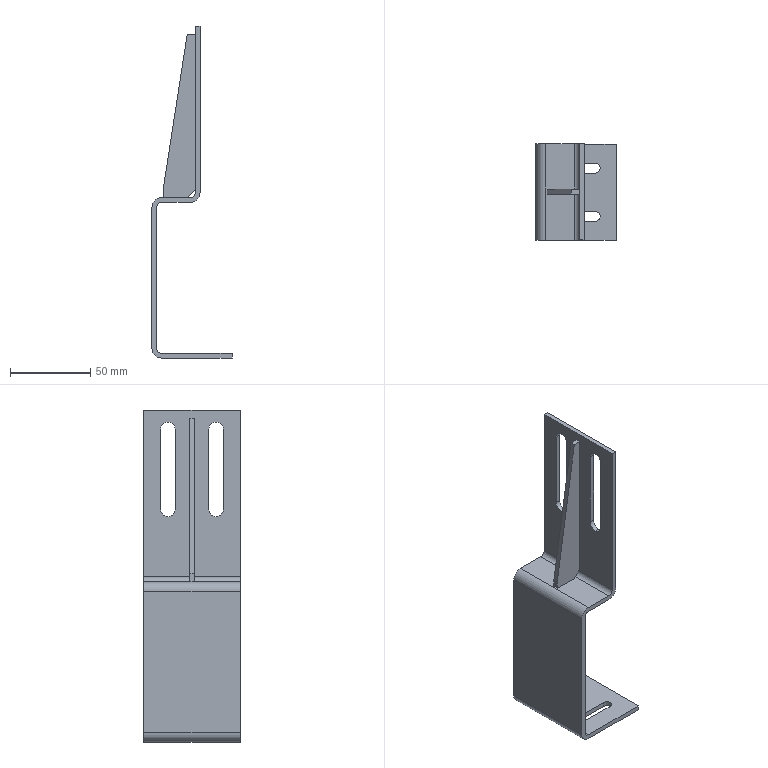Part | SolidWorks | features BaseBody 1 | 1 solid | 44 faces | box 50 x 60 x 207 mm | volume 49322 mm3 | plane 26 | cylinder 18 | commonest cylinder face diameters 6 x9 9 x6 12 x3
STEP:
#1=CARTESIAN_POINT('',(10.,15.,-97.));
#2=VERTEX_POINT('',#1);
#3=CARTESIAN_POINT('',(13.,18.,-97.));
#4=VERTEX_POINT('',#3);
#5=CARTESIAN_POINT('',(13.,15.,-97.));
#6=DIRECTION('',(0.,0.,-1.));
#7=DIRECTION('',(-1.,0.,0.));
#8=AXIS2_PLACEMENT_3D('',#5,#6,#7);
#9=CIRCLE('',#8,3.);
#10=EDGE_CURVE('',#2,#4,#9,.T.);
#11=ORIENTED_EDGE('',*,*,#10,.F.);
#12=CARTESIAN_POINT('',(10.,15.,-100.));
#13=VERTEX_POINT('',#12);
#14=CARTESIAN_POINT('',(10.,15.,-100.));
#15=DIRECTION('',(0.,0.,-1.));
#16=VECTOR('',#15,1000.);
#17=LINE('',#14,#16);
#18=EDGE_CURVE('',#2,#13,#17,.T.);
#19=ORIENTED_EDGE('',*,*,#18,.T.);
#20=CARTESIAN_POINT('',(13.,18.,-100.));
#21=VERTEX_POINT('',#20);
#22=CARTESIAN_POINT('',(13.,15.,-100.));
#23=DIRECTION('',(0.,0.,1.));
#24=DIRECTION('',(-1.,0.,0.));
#25=AXIS2_PLACEMENT_3D('',#22,#23,#24);
#26=CIRCLE('',#25,3.);
#27=EDGE_CURVE('',#21,#13,#26,.T.);
#28=ORIENTED_EDGE('',*,*,#27,.F.);
#29=CARTESIAN_POINT('',(13.,18.,-100.));
#30=DIRECTION('',(0.,0.,1.));
#31=VECTOR('',#30,1000.);
#32=LINE('',#29,#31);
#33=EDGE_CURVE('',#21,#4,#32,.T.);
#34=ORIENTED_EDGE('',*,*,#33,.T.);
#35=EDGE_LOOP('',(#11,#19,#28,#34));
#36=FACE_OUTER_BOUND('',#35,.T.);
#37=CARTESIAN_POINT('',(13.,15.,-100.));
#38=DIRECTION('',(0.,0.,-1.));
#39=DIRECTION('',(-1.,0.,0.));
#40=AXIS2_PLACEMENT_3D('',#37,#38,#39);
#41=CYLINDRICAL_SURFACE('',#40,3.);
#42=ADVANCED_FACE('',(#36),#41,.F.);
#43=CARTESIAN_POINT('',(10.,-15.,-97.));
#44=VERTEX_POINT('',#43);
#45=CARTESIAN_POINT('',(13.,-12.,-97.));
#46=VERTEX_POINT('',#45);
#47=CARTESIAN_POINT('',(13.,-15.,-97.));
#48=DIRECTION('',(0.,0.,-1.));
#49=DIRECTION('',(-1.,0.,0.));
#50=AXIS2_PLACEMENT_3D('',#47,#48,#49);
#51=CIRCLE('',#50,3.);
#52=EDGE_CURVE('',#44,#46,#51,.T.);
#53=ORIENTED_EDGE('',*,*,#52,.F.);
#54=CARTESIAN_POINT('',(10.,-15.,-100.));
#55=VERTEX_POINT('',#54);
#56=CARTESIAN_POINT('',(10.,-15.,-100.));
#57=DIRECTION('',(0.,0.,-1.));
#58=VECTOR('',#57,1000.);
#59=LINE('',#56,#58);
#60=EDGE_CURVE('',#44,#55,#59,.T.);
#61=ORIENTED_EDGE('',*,*,#60,.T.);
#62=CARTESIAN_POINT('',(13.,-12.,-100.));
#63=VERTEX_POINT('',#62);
#64=CARTESIAN_POINT('',(13.,-15.,-100.));
#65=DIRECTION('',(0.,0.,1.));
#66=DIRECTION('',(-1.,0.,0.));
#67=AXIS2_PLACEMENT_3D('',#64,#65,#66);
#68=CIRCLE('',#67,3.);
#69=EDGE_CURVE('',#63,#55,#68,.T.);
#70=ORIENTED_EDGE('',*,*,#69,.F.);
#71=CARTESIAN_POINT('',(13.,-12.,-100.));
#72=DIRECTION('',(0.,0.,-1.));
#73=VECTOR('',#72,1000.);
#74=LINE('',#71,#73);
#75=EDGE_CURVE('',#46,#63,#74,.T.);
#76=ORIENTED_EDGE('',*,*,#75,.F.);
#77=EDGE_LOOP('',(#53,#61,#70,#76));
#78=FACE_OUTER_BOUND('',#77,.T.);
#79=CARTESIAN_POINT('',(13.,-15.,-100.));
#80=DIRECTION('',(0.,0.,-1.));
#81=DIRECTION('',(-1.,0.,0.));
#82=AXIS2_PLACEMENT_3D('',#79,#80,#81);
#83=CYLINDRICAL_SURFACE('',#82,3.);
#84=ADVANCED_FACE('',(#78),#83,.F.);
#85=CARTESIAN_POINT('',(27.,15.,40.5));
#86=VERTEX_POINT('',#85);
#87=CARTESIAN_POINT('',(27.,19.5,45.));
#88=VERTEX_POINT('',#87);
#89=CARTESIAN_POINT('',(27.,15.,45.));
#90=DIRECTION('',(1.,0.,0.));
#91=DIRECTION('',(0.,0.,-1.));
#92=AXIS2_PLACEMENT_3D('',#89,#90,#91);
#93=CIRCLE('',#92,4.5);
#94=EDGE_CURVE('',#86,#88,#93,.T.);
#95=ORIENTED_EDGE('',*,*,#94,.F.);
#96=CARTESIAN_POINT('',(30.,15.,40.5));
#97=VERTEX_POINT('',#96);
#98=CARTESIAN_POINT('',(30.,15.,40.5));
#99=DIRECTION('',(1.,0.,0.));
#100=VECTOR('',#99,1000.);
#101=LINE('',#98,#100);
#102=EDGE_CURVE('',#86,#97,#101,.T.);
#103=ORIENTED_EDGE('',*,*,#102,.T.);
#104=CARTESIAN_POINT('',(30.,19.5,45.));
#105=VERTEX_POINT('',#104);
#106=CARTESIAN_POINT('',(30.,15.,45.));
#107=DIRECTION('',(-1.,0.,0.));
#108=DIRECTION('',(0.,0.,-1.));
#109=AXIS2_PLACEMENT_3D('',#106,#107,#108);
#110=CIRCLE('',#109,4.5);
#111=EDGE_CURVE('',#105,#97,#110,.T.);
#112=ORIENTED_EDGE('',*,*,#111,.F.);
#113=CARTESIAN_POINT('',(30.,19.5,45.));
#114=DIRECTION('',(-1.,0.,0.));
#115=VECTOR('',#114,1000.);
#116=LINE('',#113,#115);
#117=EDGE_CURVE('',#105,#88,#116,.T.);
#118=ORIENTED_EDGE('',*,*,#117,.T.);
#119=EDGE_LOOP('',(#95,#103,#112,#118));
#120=FACE_OUTER_BOUND('',#119,.T.);
#121=CARTESIAN_POINT('',(30.,15.,45.));
#122=DIRECTION('',(1.,0.,0.));
#123=DIRECTION('',(0.,0.,-1.));
#124=AXIS2_PLACEMENT_3D('',#121,#122,#123);
#125=CYLINDRICAL_SURFACE('',#124,4.5);
#126=ADVANCED_FACE('',(#120),#125,.F.);
#127=CARTESIAN_POINT('',(27.,-15.,40.5));
#128=VERTEX_POINT('',#127);
#129=CARTESIAN_POINT('',(27.,-10.5,45.));
#130=VERTEX_POINT('',#129);
#131=CARTESIAN_POINT('',(27.,-15.,45.));
#132=DIRECTION('',(1.,0.,0.));
#133=DIRECTION('',(0.,0.,-1.));
#134=AXIS2_PLACEMENT_3D('',#131,#132,#133);
#135=CIRCLE('',#134,4.5);
#136=EDGE_CURVE('',#128,#130,#135,.T.);
#137=ORIENTED_EDGE('',*,*,#136,.F.);
#138=CARTESIAN_POINT('',(30.,-15.,40.5));
#139=VERTEX_POINT('',#138);
#140=CARTESIAN_POINT('',(30.,-15.,40.5));
#141=DIRECTION('',(1.,0.,0.));
#142=VECTOR('',#141,1000.);
#143=LINE('',#140,#142);
#144=EDGE_CURVE('',#128,#139,#143,.T.);
#145=ORIENTED_EDGE('',*,*,#144,.T.);
#146=CARTESIAN_POINT('',(30.,-10.5,45.));
#147=VERTEX_POINT('',#146);
#148=CARTESIAN_POINT('',(30.,-15.,45.));
#149=DIRECTION('',(-1.,0.,0.));
#150=DIRECTION('',(0.,0.,-1.));
#151=AXIS2_PLACEMENT_3D('',#148,#149,#150);
#152=CIRCLE('',#151,4.5);
#153=EDGE_CURVE('',#147,#139,#152,.T.);
#154=ORIENTED_EDGE('',*,*,#153,.F.);
#155=CARTESIAN_POINT('',(30.,-10.5,45.));
#156=DIRECTION('',(1.,0.,0.));
#157=VECTOR('',#156,1000.);
#158=LINE('',#155,#157);
#159=EDGE_CURVE('',#130,#147,#158,.T.);
#160=ORIENTED_EDGE('',*,*,#159,.F.);
#161=EDGE_LOOP('',(#137,#145,#154,#160));
#162=FACE_OUTER_BOUND('',#161,.T.);
#163=CARTESIAN_POINT('',(30.,-15.,45.));
#164=DIRECTION('',(1.,0.,0.));
#165=DIRECTION('',(0.,0.,-1.));
#166=AXIS2_PLACEMENT_3D('',#163,#164,#165);
#167=CYLINDRICAL_SURFACE('',#166,4.5);
#168=ADVANCED_FACE('',(#162),#167,.F.);
#169=CARTESIAN_POINT('',(0.,30.,-94.));
#170=VERTEX_POINT('',#169);
#171=CARTESIAN_POINT('',(0.,-30.,-94.));
#172=VERTEX_POINT('',#171);
#173=CARTESIAN_POINT('',(0.,-30.,-94.));
#174=DIRECTION('',(0.,-1.,0.));
#175=VECTOR('',#174,1000.);
#176=LINE('',#173,#175);
#177=EDGE_CURVE('',#170,#172,#176,.T.);
#178=ORIENTED_EDGE('',*,*,#177,.T.);
#179=CARTESIAN_POINT('',(0.,-30.,-6.));
#180=VERTEX_POINT('',#179);
#181=CARTESIAN_POINT('',(0.,-30.,-94.));
#182=DIRECTION('',(0.,0.,1.));
#183=VECTOR('',#182,1000.);
#184=LINE('',#181,#183);
#185=EDGE_CURVE('',#172,#180,#184,.T.);
#186=ORIENTED_EDGE('',*,*,#185,.T.);
#187=CARTESIAN_POINT('',(0.,30.,-6.));
#188=VERTEX_POINT('',#187);
#189=CARTESIAN_POINT('',(0.,-30.,-6.));
#190=DIRECTION('',(0.,1.,0.));
#191=VECTOR('',#190,1000.);
#192=LINE('',#189,#191);
#193=EDGE_CURVE('',#180,#188,#192,.T.);
#194=ORIENTED_EDGE('',*,*,#193,.T.);
#195=CARTESIAN_POINT('',(0.,30.,-94.));
#196=DIRECTION('',(0.,0.,-1.));
#197=VECTOR('',#196,1000.);
#198=LINE('',#195,#197);
#199=EDGE_CURVE('',#188,#170,#198,.T.);
#200=ORIENTED_EDGE('',*,*,#199,.T.);
#201=EDGE_LOOP('',(#178,#186,#194,#200));
#202=FACE_OUTER_BOUND('',#201,.T.);
#203=CARTESIAN_POINT('',(0.,-30.,-94.));
#204=DIRECTION('',(-1.,0.,0.));
#205=DIRECTION('',(0.,0.,1.));
#206=AXIS2_PLACEMENT_3D('',#203,#204,#205);
#207=PLANE('',#206);
#208=ADVANCED_FACE('',(#202),#207,.T.);
#209=CARTESIAN_POINT('',(6.,-30.,-100.));
#210=VERTEX_POINT('',#209);
#211=CARTESIAN_POINT('',(6.,-30.,-94.));
#212=DIRECTION('',(0.,1.,0.));
#213=DIRECTION('',(0.,0.,1.));
#214=AXIS2_PLACEMENT_3D('',#211,#212,#213);
#215=CIRCLE('',#214,6.);
#216=EDGE_CURVE('',#210,#172,#215,.T.);
#217=ORIENTED_EDGE('',*,*,#216,.F.);
#218=CARTESIAN_POINT('',(50.,-30.,-100.));
#219=VERTEX_POINT('',#218);
#220=CARTESIAN_POINT('',(0.,-30.,-100.));
#221=DIRECTION('',(-1.,0.,0.));
#222=VECTOR('',#221,1000.);
#223=LINE('',#220,#222);
#224=EDGE_CURVE('',#219,#210,#223,.T.);
#225=ORIENTED_EDGE('',*,*,#224,.F.);
#226=CARTESIAN_POINT('',(50.,-30.,-97.));
#227=VERTEX_POINT('',#226);
#228=CARTESIAN_POINT('',(50.,-30.,0.));
#229=DIRECTION('',(0.,0.,-1.));
#230=VECTOR('',#229,1000.);
#231=LINE('',#228,#230);
#232=EDGE_CURVE('',#227,#219,#231,.T.);
#233=ORIENTED_EDGE('',*,*,#232,.F.);
#234=CARTESIAN_POINT('',(6.,-30.,-97.));
#235=VERTEX_POINT('',#234);
#236=CARTESIAN_POINT('',(0.,-30.,-97.));
#237=DIRECTION('',(1.,0.,0.));
#238=VECTOR('',#237,1000.);
#239=LINE('',#236,#238);
#240=EDGE_CURVE('',#235,#227,#239,.T.);
#241=ORIENTED_EDGE('',*,*,#240,.F.);
#242=CARTESIAN_POINT('',(3.,-30.,-94.));
#243=VERTEX_POINT('',#242);
#244=CARTESIAN_POINT('',(6.,-30.,-94.));
#245=DIRECTION('',(0.,-1.,0.));
#246=DIRECTION('',(0.,0.,1.));
#247=AXIS2_PLACEMENT_3D('',#244,#245,#246);
#248=CIRCLE('',#247,3.);
#249=EDGE_CURVE('',#243,#235,#248,.T.);
#250=ORIENTED_EDGE('',*,*,#249,.F.);
#251=CARTESIAN_POINT('',(3.,-30.,-6.));
#252=VERTEX_POINT('',#251);
#253=CARTESIAN_POINT('',(3.,-30.,0.));
#254=DIRECTION('',(0.,0.,-1.));
#255=VECTOR('',#254,1000.);
#256=LINE('',#253,#255);
#257=EDGE_CURVE('',#252,#243,#256,.T.);
#258=ORIENTED_EDGE('',*,*,#257,.F.);
#259=CARTESIAN_POINT('',(6.,-30.,-3.));
#260=VERTEX_POINT('',#259);
#261=CARTESIAN_POINT('',(6.,-30.,-6.));
#262=DIRECTION('',(0.,-1.,0.));
#263=DIRECTION('',(0.,0.,1.));
#264=AXIS2_PLACEMENT_3D('',#261,#262,#263);
#265=CIRCLE('',#264,3.);
#266=EDGE_CURVE('',#260,#252,#265,.T.);
#267=ORIENTED_EDGE('',*,*,#266,.F.);
#268=CARTESIAN_POINT('',(24.,-30.,-3.));
#269=VERTEX_POINT('',#268);
#270=CARTESIAN_POINT('',(0.,-30.,-3.));
#271=DIRECTION('',(-1.,0.,0.));
#272=VECTOR('',#271,1000.);
#273=LINE('',#270,#272);
#274=EDGE_CURVE('',#269,#260,#273,.T.);
#275=ORIENTED_EDGE('',*,*,#274,.F.);
#276=CARTESIAN_POINT('',(30.,-30.,3.));
#277=VERTEX_POINT('',#276);
#278=CARTESIAN_POINT('',(24.,-30.,3.));
#279=DIRECTION('',(0.,1.,0.));
#280=DIRECTION('',(0.,0.,1.));
#281=AXIS2_PLACEMENT_3D('',#278,#279,#280);
#282=CIRCLE('',#281,6.);
#283=EDGE_CURVE('',#277,#269,#282,.T.);
#284=ORIENTED_EDGE('',*,*,#283,.F.);
#285=CARTESIAN_POINT('',(30.,-30.,107.));
#286=VERTEX_POINT('',#285);
#287=CARTESIAN_POINT('',(30.,-30.,0.));
#288=DIRECTION('',(0.,0.,-1.));
#289=VECTOR('',#288,1000.);
#290=LINE('',#287,#289);
#291=EDGE_CURVE('',#286,#277,#290,.T.);
#292=ORIENTED_EDGE('',*,*,#291,.F.);
#293=CARTESIAN_POINT('',(27.,-30.,107.));
#294=VERTEX_POINT('',#293);
#295=CARTESIAN_POINT('',(0.,-30.,107.));
#296=DIRECTION('',(1.,0.,0.));
#297=VECTOR('',#296,1000.);
#298=LINE('',#295,#297);
#299=EDGE_CURVE('',#294,#286,#298,.T.);
#300=ORIENTED_EDGE('',*,*,#299,.F.);
#301=CARTESIAN_POINT('',(27.,-30.,3.));
#302=VERTEX_POINT('',#301);
#303=CARTESIAN_POINT('',(27.,-30.,0.));
#304=DIRECTION('',(0.,0.,1.));
#305=VECTOR('',#304,1000.);
#306=LINE('',#303,#305);
#307=EDGE_CURVE('',#302,#294,#306,.T.);
#308=ORIENTED_EDGE('',*,*,#307,.F.);
#309=CARTESIAN_POINT('',(24.,-30.,0.));
#310=VERTEX_POINT('',#309);
#311=CARTESIAN_POINT('',(24.,-30.,3.));
#312=DIRECTION('',(0.,-1.,0.));
#313=DIRECTION('',(0.,0.,1.));
#314=AXIS2_PLACEMENT_3D('',#311,#312,#313);
#315=CIRCLE('',#314,3.);
#316=EDGE_CURVE('',#310,#302,#315,.T.);
#317=ORIENTED_EDGE('',*,*,#316,.F.);
#318=CARTESIAN_POINT('',(6.,-30.,0.));
#319=VERTEX_POINT('',#318);
#320=CARTESIAN_POINT('',(0.,-30.,0.));
#321=DIRECTION('',(1.,0.,0.));
#322=VECTOR('',#321,1000.);
#323=LINE('',#320,#322);
#324=EDGE_CURVE('',#319,#310,#323,.T.);
#325=ORIENTED_EDGE('',*,*,#324,.F.);
#326=CARTESIAN_POINT('',(6.,-30.,-6.));
#327=DIRECTION('',(0.,1.,0.));
#328=DIRECTION('',(0.,0.,1.));
#329=AXIS2_PLACEMENT_3D('',#326,#327,#328);
#330=CIRCLE('',#329,6.);
#331=EDGE_CURVE('',#180,#319,#330,.T.);
#332=ORIENTED_EDGE('',*,*,#331,.F.);
#333=ORIENTED_EDGE('',*,*,#185,.F.);
#334=EDGE_LOOP('',(#217,#225,#233,#241,#250,#258,#267,#275,#284,#292,#300,#308,#317,#325,#332,#333));
#335=FACE_OUTER_BOUND('',#334,.T.);
#336=CARTESIAN_POINT('',(0.,-30.,0.));
#337=DIRECTION('',(0.,1.,0.));
#338=DIRECTION('',(0.,0.,1.));
#339=AXIS2_PLACEMENT_3D('',#336,#337,#338);
#340=PLANE('',#339);
#341=ADVANCED_FACE('',(#335),#340,.F.);
#342=CARTESIAN_POINT('',(6.,30.,-100.));
#343=VERTEX_POINT('',#342);
#344=CARTESIAN_POINT('',(6.,-30.,-100.));
#345=DIRECTION('',(0.,-1.,0.));
#346=VECTOR('',#345,1000.);
#347=LINE('',#344,#346);
#348=EDGE_CURVE('',#343,#210,#347,.T.);
#349=ORIENTED_EDGE('',*,*,#348,.T.);
#350=ORIENTED_EDGE('',*,*,#216,.T.);
#351=ORIENTED_EDGE('',*,*,#177,.F.);
#352=CARTESIAN_POINT('',(6.,30.,-94.));
#353=DIRECTION('',(0.,-1.,0.));
#354=DIRECTION('',(0.,0.,1.));
#355=AXIS2_PLACEMENT_3D('',#352,#353,#354);
#356=CIRCLE('',#355,6.);
#357=EDGE_CURVE('',#170,#343,#356,.T.);
#358=ORIENTED_EDGE('',*,*,#357,.T.);
#359=EDGE_LOOP('',(#349,#350,#351,#358));
#360=FACE_OUTER_BOUND('',#359,.T.);
#361=CARTESIAN_POINT('',(6.,-30.,-94.));
#362=DIRECTION('',(0.,1.,0.));
#363=DIRECTION('',(0.,0.,1.));
#364=AXIS2_PLACEMENT_3D('',#361,#362,#363);
#365=CYLINDRICAL_SURFACE('',#364,6.);
#366=ADVANCED_FACE('',(#360),#365,.T.);
#367=ORIENTED_EDGE('',*,*,#199,.F.);
#368=CARTESIAN_POINT('',(6.,30.,0.));
#369=VERTEX_POINT('',#368);
#370=CARTESIAN_POINT('',(6.,30.,-6.));
#371=DIRECTION('',(0.,1.,0.));
#372=DIRECTION('',(0.,0.,1.));
#373=AXIS2_PLACEMENT_3D('',#370,#371,#372);
#374=CIRCLE('',#373,6.);
#375=EDGE_CURVE('',#188,#369,#374,.T.);
#376=ORIENTED_EDGE('',*,*,#375,.T.);
#377=CARTESIAN_POINT('',(24.,30.,0.));
#378=VERTEX_POINT('',#377);
#379=CARTESIAN_POINT('',(0.,30.,0.));
#380=DIRECTION('',(1.,0.,0.));
#381=VECTOR('',#380,1000.);
#382=LINE('',#379,#381);
#383=EDGE_CURVE('',#369,#378,#382,.T.);
#384=ORIENTED_EDGE('',*,*,#383,.T.);
#385=CARTESIAN_POINT('',(27.,30.,3.));
#386=VERTEX_POINT('',#385);
#387=CARTESIAN_POINT('',(24.,30.,3.));
#388=DIRECTION('',(0.,-1.,0.));
#389=DIRECTION('',(0.,0.,1.));
#390=AXIS2_PLACEMENT_3D('',#387,#388,#389);
#391=CIRCLE('',#390,3.);
#392=EDGE_CURVE('',#378,#386,#391,.T.);
#393=ORIENTED_EDGE('',*,*,#392,.T.);
#394=CARTESIAN_POINT('',(27.,30.,107.));
#395=VERTEX_POINT('',#394);
#396=CARTESIAN_POINT('',(27.,30.,0.));
#397=DIRECTION('',(0.,0.,1.));
#398=VECTOR('',#397,1000.);
#399=LINE('',#396,#398);
#400=EDGE_CURVE('',#386,#395,#399,.T.);
#401=ORIENTED_EDGE('',*,*,#400,.T.);
#402=CARTESIAN_POINT('',(30.,30.,107.));
#403=VERTEX_POINT('',#402);
#404=CARTESIAN_POINT('',(0.,30.,107.));
#405=DIRECTION('',(1.,0.,0.));
#406=VECTOR('',#405,1000.);
#407=LINE('',#404,#406);
#408=EDGE_CURVE('',#395,#403,#407,.T.);
#409=ORIENTED_EDGE('',*,*,#408,.T.);
#410=CARTESIAN_POINT('',(30.,30.,3.));
#411=VERTEX_POINT('',#410);
#412=CARTESIAN_POINT('',(30.,30.,0.));
#413=DIRECTION('',(0.,0.,-1.));
#414=VECTOR('',#413,1000.);
#415=LINE('',#412,#414);
#416=EDGE_CURVE('',#403,#411,#415,.T.);
#417=ORIENTED_EDGE('',*,*,#416,.T.);
#418=CARTESIAN_POINT('',(24.,30.,-3.));
#419=VERTEX_POINT('',#418);
#420=CARTESIAN_POINT('',(24.,30.,3.));
#421=DIRECTION('',(0.,1.,0.));
#422=DIRECTION('',(0.,0.,1.));
#423=AXIS2_PLACEMENT_3D('',#420,#421,#422);
#424=CIRCLE('',#423,6.);
#425=EDGE_CURVE('',#411,#419,#424,.T.);
#426=ORIENTED_EDGE('',*,*,#425,.T.);
#427=CARTESIAN_POINT('',(6.,30.,-3.));
#428=VERTEX_POINT('',#427);
#429=CARTESIAN_POINT('',(0.,30.,-3.));
#430=DIRECTION('',(-1.,0.,0.));
#431=VECTOR('',#430,1000.);
#432=LINE('',#429,#431);
#433=EDGE_CURVE('',#419,#428,#432,.T.);
#434=ORIENTED_EDGE('',*,*,#433,.T.);
#435=CARTESIAN_POINT('',(3.,30.,-6.));
#436=VERTEX_POINT('',#435);
#437=CARTESIAN_POINT('',(6.,30.,-6.));
#438=DIRECTION('',(0.,-1.,0.));
#439=DIRECTION('',(0.,0.,1.));
#440=AXIS2_PLACEMENT_3D('',#437,#438,#439);
#441=CIRCLE('',#440,3.);
#442=EDGE_CURVE('',#428,#436,#441,.T.);
#443=ORIENTED_EDGE('',*,*,#442,.T.);
#444=CARTESIAN_POINT('',(3.,30.,-94.));
#445=VERTEX_POINT('',#444);
#446=CARTESIAN_POINT('',(3.,30.,0.));
#447=DIRECTION('',(0.,0.,-1.));
#448=VECTOR('',#447,1000.);
#449=LINE('',#446,#448);
#450=EDGE_CURVE('',#436,#445,#449,.T.);
#451=ORIENTED_EDGE('',*,*,#450,.T.);
#452=CARTESIAN_POINT('',(6.,30.,-97.));
#453=VERTEX_POINT('',#452);
#454=CARTESIAN_POINT('',(6.,30.,-94.));
#455=DIRECTION('',(0.,-1.,0.));
#456=DIRECTION('',(0.,0.,1.));
#457=AXIS2_PLACEMENT_3D('',#454,#455,#456);
#458=CIRCLE('',#457,3.);
#459=EDGE_CURVE('',#445,#453,#458,.T.);
#460=ORIENTED_EDGE('',*,*,#459,.T.);
#461=CARTESIAN_POINT('',(50.,30.,-97.));
#462=VERTEX_POINT('',#461);
#463=CARTESIAN_POINT('',(0.,30.,-97.));
#464=DIRECTION('',(1.,0.,0.));
#465=VECTOR('',#464,1000.);
#466=LINE('',#463,#465);
#467=EDGE_CURVE('',#453,#462,#466,.T.);
#468=ORIENTED_EDGE('',*,*,#467,.T.);
#469=CARTESIAN_POINT('',(50.,30.,-100.));
#470=VERTEX_POINT('',#469);
#471=CARTESIAN_POINT('',(50.,30.,0.));
#472=DIRECTION('',(0.,0.,-1.));
#473=VECTOR('',#472,1000.);
#474=LINE('',#471,#473);
#475=EDGE_CURVE('',#462,#470,#474,.T.);
#476=ORIENTED_EDGE('',*,*,#475,.T.);
#477=CARTESIAN_POINT('',(0.,30.,-100.));
#478=DIRECTION('',(-1.,0.,0.));
#479=VECTOR('',#478,1000.);
#480=LINE('',#477,#479);
#481=EDGE_CURVE('',#470,#343,#480,.T.);
#482=ORIENTED_EDGE('',*,*,#481,.T.);
#483=ORIENTED_EDGE('',*,*,#357,.F.);
#484=EDGE_LOOP('',(#367,#376,#384,#393,#401,#409,#417,#426,#434,#443,#451,#460,#468,#476,#482,#483));
#485=FACE_OUTER_BOUND('',#484,.T.);
#486=CARTESIAN_POINT('',(0.,30.,0.));
#487=DIRECTION('',(0.,1.,0.));
#488=DIRECTION('',(0.,0.,1.));
#489=AXIS2_PLACEMENT_3D('',#486,#487,#488);
#490=PLANE('',#489);
#491=ADVANCED_FACE('',(#485),#490,.T.);
#492=ORIENTED_EDGE('',*,*,#193,.F.);
#493=ORIENTED_EDGE('',*,*,#331,.T.);
#494=CARTESIAN_POINT('',(6.,-30.,0.));
#495=DIRECTION('',(0.,1.,0.));
#496=VECTOR('',#495,1000.);
#497=LINE('',#494,#496);
#498=EDGE_CURVE('',#319,#369,#497,.T.);
#499=ORIENTED_EDGE('',*,*,#498,.T.);
#500=ORIENTED_EDGE('',*,*,#375,.F.);
#501=EDGE_LOOP('',(#492,#493,#499,#500));
#502=FACE_OUTER_BOUND('',#501,.T.);
#503=CARTESIAN_POINT('',(6.,-30.,-6.));
#504=DIRECTION('',(0.,1.,0.));
#505=DIRECTION('',(0.,0.,1.));
#506=AXIS2_PLACEMENT_3D('',#503,#504,#505);
#507=CYLINDRICAL_SURFACE('',#506,6.);
#508=ADVANCED_FACE('',(#502),#507,.T.);
#509=CARTESIAN_POINT('',(37.,12.,-100.));
#510=VERTEX_POINT('',#509);
#511=CARTESIAN_POINT('',(37.,18.,-100.));
#512=VERTEX_POINT('',#511);
#513=CARTESIAN_POINT('',(37.,15.,-100.));
#514=DIRECTION('',(0.,0.,1.));
#515=DIRECTION('',(-1.,0.,0.));
#516=AXIS2_PLACEMENT_3D('',#513,#514,#515);
#517=CIRCLE('',#516,3.);
#518=EDGE_CURVE('',#510,#512,#517,.T.);
#519=ORIENTED_EDGE('',*,*,#518,.T.);
#520=CARTESIAN_POINT('',(50.,18.,-100.));
#521=DIRECTION('',(-1.,0.,0.));
#522=VECTOR('',#521,1000.);
#523=LINE('',#520,#522);
#524=EDGE_CURVE('',#512,#21,#523,.T.);
#525=ORIENTED_EDGE('',*,*,#524,.T.);
#526=ORIENTED_EDGE('',*,*,#27,.T.);
#527=CARTESIAN_POINT('',(13.,12.,-100.));
#528=VERTEX_POINT('',#527);
#529=CARTESIAN_POINT('',(13.,15.,-100.));
#530=DIRECTION('',(0.,0.,1.));
#531=DIRECTION('',(-1.,0.,0.));
#532=AXIS2_PLACEMENT_3D('',#529,#530,#531);
#533=CIRCLE('',#532,3.);
#534=EDGE_CURVE('',#13,#528,#533,.T.);
#535=ORIENTED_EDGE('',*,*,#534,.T.);
#536=CARTESIAN_POINT('',(50.,12.,-100.));
#537=DIRECTION('',(1.,0.,0.));
#538=VECTOR('',#537,1000.);
#539=LINE('',#536,#538);
#540=EDGE_CURVE('',#528,#510,#539,.T.);
#541=ORIENTED_EDGE('',*,*,#540,.T.);
#542=EDGE_LOOP('',(#519,#525,#526,#535,#541));
#543=FACE_BOUND('',#542,.T.);
#544=CARTESIAN_POINT('',(37.,-12.,-100.));
#545=VERTEX_POINT('',#544);
#546=CARTESIAN_POINT('',(50.,-12.,-100.));
#547=DIRECTION('',(-1.,0.,0.));
#548=VECTOR('',#547,1000.);
#549=LINE('',#546,#548);
#550=EDGE_CURVE('',#545,#63,#549,.T.);
#551=ORIENTED_EDGE('',*,*,#550,.T.);
#552=ORIENTED_EDGE('',*,*,#69,.T.);
#553=CARTESIAN_POINT('',(13.,-18.,-100.));
#554=VERTEX_POINT('',#553);
#555=CARTESIAN_POINT('',(13.,-15.,-100.));
#556=DIRECTION('',(0.,0.,1.));
#557=DIRECTION('',(-1.,0.,0.));
#558=AXIS2_PLACEMENT_3D('',#555,#556,#557);
#559=CIRCLE('',#558,3.);
#560=EDGE_CURVE('',#55,#554,#559,.T.);
#561=ORIENTED_EDGE('',*,*,#560,.T.);
#562=CARTESIAN_POINT('',(37.,-18.,-100.));
#563=VERTEX_POINT('',#562);
#564=CARTESIAN_POINT('',(50.,-18.,-100.));
#565=DIRECTION('',(1.,0.,0.));
#566=VECTOR('',#565,1000.);
#567=LINE('',#564,#566);
#568=EDGE_CURVE('',#554,#563,#567,.T.);
#569=ORIENTED_EDGE('',*,*,#568,.T.);
#570=CARTESIAN_POINT('',(37.,-15.,-100.));
#571=DIRECTION('',(0.,0.,1.));
#572=DIRECTION('',(-1.,0.,0.));
#573=AXIS2_PLACEMENT_3D('',#570,#571,#572);
#574=CIRCLE('',#573,3.);
#575=EDGE_CURVE('',#563,#545,#574,.T.);
#576=ORIENTED_EDGE('',*,*,#575,.T.);
#577=EDGE_LOOP('',(#551,#552,#561,#569,#576));
#578=FACE_BOUND('',#577,.T.);
#579=CARTESIAN_POINT('',(50.,-30.,-100.));
#580=DIRECTION('',(0.,-1.,0.));
#581=VECTOR('',#580,1000.);
#582=LINE('',#579,#581);
#583=EDGE_CURVE('',#470,#219,#582,.T.);
#584=ORIENTED_EDGE('',*,*,#583,.T.);
#585=ORIENTED_EDGE('',*,*,#224,.T.);
#586=ORIENTED_EDGE('',*,*,#348,.F.);
#587=ORIENTED_EDGE('',*,*,#481,.F.);
#588=EDGE_LOOP('',(#584,#585,#586,#587));
#589=FACE_OUTER_BOUND('',#588,.T.);
#590=CARTESIAN_POINT('',(50.,-30.,-100.));
#591=DIRECTION('',(0.,0.,-1.));
#592=DIRECTION('',(-1.,0.,0.));
#593=AXIS2_PLACEMENT_3D('',#590,#591,#592);
#594=PLANE('',#593);
#595=ADVANCED_FACE('',(#543,#578,#589),#594,.T.);
#596=CARTESIAN_POINT('',(50.,-30.,-97.));
#597=DIRECTION('',(0.,-1.,0.));
#598=VECTOR('',#597,1000.);
#599=LINE('',#596,#598);
#600=EDGE_CURVE('',#462,#227,#599,.T.);
#601=ORIENTED_EDGE('',*,*,#600,.T.);
#602=ORIENTED_EDGE('',*,*,#232,.T.);
#603=ORIENTED_EDGE('',*,*,#583,.F.);
#604=ORIENTED_EDGE('',*,*,#475,.F.);
#605=EDGE_LOOP('',(#601,#602,#603,#604));
#606=FACE_OUTER_BOUND('',#605,.T.);
#607=CARTESIAN_POINT('',(50.,-30.,-97.));
#608=DIRECTION('',(1.,0.,0.));
#609=DIRECTION('',(0.,0.,-1.));
#610=AXIS2_PLACEMENT_3D('',#607,#608,#609);
#611=PLANE('',#610);
#612=ADVANCED_FACE('',(#606),#611,.T.);
#613=CARTESIAN_POINT('',(13.,12.,-97.));
#614=VERTEX_POINT('',#613);
#615=CARTESIAN_POINT('',(13.,15.,-97.));
#616=DIRECTION('',(0.,0.,-1.));
#617=DIRECTION('',(-1.,0.,0.));
#618=AXIS2_PLACEMENT_3D('',#615,#616,#617);
#619=CIRCLE('',#618,3.);
#620=EDGE_CURVE('',#614,#2,#619,.T.);
#621=ORIENTED_EDGE('',*,*,#620,.T.);
#622=ORIENTED_EDGE('',*,*,#10,.T.);
#623=CARTESIAN_POINT('',(37.,18.,-97.));
#624=VERTEX_POINT('',#623);
#625=CARTESIAN_POINT('',(6.,18.,-97.));
#626=DIRECTION('',(1.,0.,0.));
#627=VECTOR('',#626,1000.);
#628=LINE('',#625,#627);
#629=EDGE_CURVE('',#4,#624,#628,.T.);
#630=ORIENTED_EDGE('',*,*,#629,.T.);
#631=CARTESIAN_POINT('',(37.,12.,-97.));
#632=VERTEX_POINT('',#631);
#633=CARTESIAN_POINT('',(37.,15.,-97.));
#634=DIRECTION('',(0.,0.,-1.));
#635=DIRECTION('',(-1.,0.,0.));
#636=AXIS2_PLACEMENT_3D('',#633,#634,#635);
#637=CIRCLE('',#636,3.);
#638=EDGE_CURVE('',#624,#632,#637,.T.);
#639=ORIENTED_EDGE('',*,*,#638,.T.);
#640=CARTESIAN_POINT('',(6.,12.,-97.));
#641=DIRECTION('',(-1.,0.,0.));
#642=VECTOR('',#641,1000.);
#643=LINE('',#640,#642);
#644=EDGE_CURVE('',#632,#614,#643,.T.);
#645=ORIENTED_EDGE('',*,*,#644,.T.);
#646=EDGE_LOOP('',(#621,#622,#630,#639,#645));
#647=FACE_BOUND('',#646,.T.);
#648=CARTESIAN_POINT('',(37.,-18.,-97.));
#649=VERTEX_POINT('',#648);
#650=CARTESIAN_POINT('',(13.,-18.,-97.));
#651=VERTEX_POINT('',#650);
#652=CARTESIAN_POINT('',(6.,-18.,-97.));
#653=DIRECTION('',(-1.,0.,0.));
#654=VECTOR('',#653,1000.);
#655=LINE('',#652,#654);
#656=EDGE_CURVE('',#649,#651,#655,.T.);
#657=ORIENTED_EDGE('',*,*,#656,.T.);
#658=CARTESIAN_POINT('',(13.,-15.,-97.));
#659=DIRECTION('',(0.,0.,-1.));
#660=DIRECTION('',(-1.,0.,0.));
#661=AXIS2_PLACEMENT_3D('',#658,#659,#660);
#662=CIRCLE('',#661,3.);
#663=EDGE_CURVE('',#651,#44,#662,.T.);
#664=ORIENTED_EDGE('',*,*,#663,.T.);
#665=ORIENTED_EDGE('',*,*,#52,.T.);
#666=CARTESIAN_POINT('',(37.,-12.,-97.));
#667=VERTEX_POINT('',#666);
#668=CARTESIAN_POINT('',(6.,-12.,-97.));
#669=DIRECTION('',(1.,0.,0.));
#670=VECTOR('',#669,1000.);
#671=LINE('',#668,#670);
#672=EDGE_CURVE('',#46,#667,#671,.T.);
#673=ORIENTED_EDGE('',*,*,#672,.T.);
#674=CARTESIAN_POINT('',(37.,-15.,-97.));
#675=DIRECTION('',(0.,0.,-1.));
#676=DIRECTION('',(-1.,0.,0.));
#677=AXIS2_PLACEMENT_3D('',#674,#675,#676);
#678=CIRCLE('',#677,3.);
#679=EDGE_CURVE('',#667,#649,#678,.T.);
#680=ORIENTED_EDGE('',*,*,#679,.T.);
#681=EDGE_LOOP('',(#657,#664,#665,#673,#680));
#682=FACE_BOUND('',#681,.T.);
#683=CARTESIAN_POINT('',(6.,-30.,-97.));
#684=DIRECTION('',(0.,-1.,0.));
#685=VECTOR('',#684,1000.);
#686=LINE('',#683,#685);
#687=EDGE_CURVE('',#453,#235,#686,.T.);
#688=ORIENTED_EDGE('',*,*,#687,.T.);
#689=ORIENTED_EDGE('',*,*,#240,.T.);
#690=ORIENTED_EDGE('',*,*,#600,.F.);
#691=ORIENTED_EDGE('',*,*,#467,.F.);
#692=EDGE_LOOP('',(#688,#689,#690,#691));
#693=FACE_OUTER_BOUND('',#692,.T.);
#694=CARTESIAN_POINT('',(6.,-30.,-97.));
#695=DIRECTION('',(0.,0.,1.));
#696=DIRECTION('',(1.,0.,0.));
#697=AXIS2_PLACEMENT_3D('',#694,#695,#696);
#698=PLANE('',#697);
#699=ADVANCED_FACE('',(#647,#682,#693),#698,.T.);
#700=ORIENTED_EDGE('',*,*,#459,.F.);
#701=CARTESIAN_POINT('',(3.,-30.,-94.));
#702=DIRECTION('',(0.,1.,0.));
#703=VECTOR('',#702,1000.);
#704=LINE('',#701,#703);
#705=EDGE_CURVE('',#243,#445,#704,.T.);
#706=ORIENTED_EDGE('',*,*,#705,.F.);
#707=ORIENTED_EDGE('',*,*,#249,.T.);
#708=ORIENTED_EDGE('',*,*,#687,.F.);
#709=EDGE_LOOP('',(#700,#706,#707,#708));
#710=FACE_OUTER_BOUND('',#709,.T.);
#711=CARTESIAN_POINT('',(6.,-30.,-94.));
#712=DIRECTION('',(0.,1.,0.));
#713=DIRECTION('',(0.,0.,1.));
#714=AXIS2_PLACEMENT_3D('',#711,#712,#713);
#715=CYLINDRICAL_SURFACE('',#714,3.);
#716=ADVANCED_FACE('',(#710),#715,.F.);
#717=CARTESIAN_POINT('',(3.,-30.,-6.));
#718=DIRECTION('',(0.,-1.,0.));
#719=VECTOR('',#718,1000.);
#720=LINE('',#717,#719);
#721=EDGE_CURVE('',#436,#252,#720,.T.);
#722=ORIENTED_EDGE('',*,*,#721,.T.);
#723=ORIENTED_EDGE('',*,*,#257,.T.);
#724=ORIENTED_EDGE('',*,*,#705,.T.);
#725=ORIENTED_EDGE('',*,*,#450,.F.);
#726=EDGE_LOOP('',(#722,#723,#724,#725));
#727=FACE_OUTER_BOUND('',#726,.T.);
#728=CARTESIAN_POINT('',(3.,-30.,-6.));
#729=DIRECTION('',(1.,0.,0.));
#730=DIRECTION('',(0.,0.,-1.));
#731=AXIS2_PLACEMENT_3D('',#728,#729,#730);
#732=PLANE('',#731);
#733=ADVANCED_FACE('',(#727),#732,.T.);
#734=ORIENTED_EDGE('',*,*,#442,.F.);
#735=CARTESIAN_POINT('',(6.,-30.,-3.));
#736=DIRECTION('',(0.,1.,0.));
#737=VECTOR('',#736,1000.);
#738=LINE('',#735,#737);
#739=EDGE_CURVE('',#260,#428,#738,.T.);
#740=ORIENTED_EDGE('',*,*,#739,.F.);
#741=ORIENTED_EDGE('',*,*,#266,.T.);
#742=ORIENTED_EDGE('',*,*,#721,.F.);
#743=EDGE_LOOP('',(#734,#740,#741,#742));
#744=FACE_OUTER_BOUND('',#743,.T.);
#745=CARTESIAN_POINT('',(6.,-30.,-6.));
#746=DIRECTION('',(0.,1.,0.));
#747=DIRECTION('',(0.,0.,1.));
#748=AXIS2_PLACEMENT_3D('',#745,#746,#747);
#749=CYLINDRICAL_SURFACE('',#748,3.);
#750=ADVANCED_FACE('',(#744),#749,.F.);
#751=CARTESIAN_POINT('',(24.,-30.,-3.));
#752=DIRECTION('',(0.,-1.,0.));
#753=VECTOR('',#752,1000.);
#754=LINE('',#751,#753);
#755=EDGE_CURVE('',#419,#269,#754,.T.);
#756=ORIENTED_EDGE('',*,*,#755,.T.);
#757=ORIENTED_EDGE('',*,*,#274,.T.);
#758=ORIENTED_EDGE('',*,*,#739,.T.);
#759=ORIENTED_EDGE('',*,*,#433,.F.);
#760=EDGE_LOOP('',(#756,#757,#758,#759));
#761=FACE_OUTER_BOUND('',#760,.T.);
#762=CARTESIAN_POINT('',(24.,-30.,-3.));
#763=DIRECTION('',(0.,0.,-1.));
#764=DIRECTION('',(-1.,0.,0.));
#765=AXIS2_PLACEMENT_3D('',#762,#763,#764);
#766=PLANE('',#765);
#767=ADVANCED_FACE('',(#761),#766,.T.);
#768=CARTESIAN_POINT('',(30.,-30.,3.));
#769=DIRECTION('',(0.,-1.,0.));
#770=VECTOR('',#769,1000.);
#771=LINE('',#768,#770);
#772=EDGE_CURVE('',#411,#277,#771,.T.);
#773=ORIENTED_EDGE('',*,*,#772,.T.);
#774=ORIENTED_EDGE('',*,*,#283,.T.);
#775=ORIENTED_EDGE('',*,*,#755,.F.);
#776=ORIENTED_EDGE('',*,*,#425,.F.);
#777=EDGE_LOOP('',(#773,#774,#775,#776));
#778=FACE_OUTER_BOUND('',#777,.T.);
#779=CARTESIAN_POINT('',(24.,-30.,3.));
#780=DIRECTION('',(0.,1.,0.));
#781=DIRECTION('',(0.,0.,1.));
#782=AXIS2_PLACEMENT_3D('',#779,#780,#781);
#783=CYLINDRICAL_SURFACE('',#782,6.);
#784=ADVANCED_FACE('',(#778),#783,.T.);
#785=CARTESIAN_POINT('',(30.,10.5,95.));
#786=VERTEX_POINT('',#785);
#787=CARTESIAN_POINT('',(30.,19.5,95.));
#788=VERTEX_POINT('',#787);
#789=CARTESIAN_POINT('',(30.,15.,95.));
#790=DIRECTION('',(-1.,0.,0.));
#791=DIRECTION('',(0.,0.,-1.));
#792=AXIS2_PLACEMENT_3D('',#789,#790,#791);
#793=CIRCLE('',#792,4.5);
#794=EDGE_CURVE('',#786,#788,#793,.T.);
#795=ORIENTED_EDGE('',*,*,#794,.T.);
#796=CARTESIAN_POINT('',(30.,19.5,107.));
#797=DIRECTION('',(0.,0.,-1.));
#798=VECTOR('',#797,1000.);
#799=LINE('',#796,#798);
#800=EDGE_CURVE('',#788,#105,#799,.T.);
#801=ORIENTED_EDGE('',*,*,#800,.T.);
#802=ORIENTED_EDGE('',*,*,#111,.T.);
#803=CARTESIAN_POINT('',(30.,10.5,45.));
#804=VERTEX_POINT('',#803);
#805=CARTESIAN_POINT('',(30.,15.,45.));
#806=DIRECTION('',(-1.,0.,0.));
#807=DIRECTION('',(0.,0.,-1.));
#808=AXIS2_PLACEMENT_3D('',#805,#806,#807);
#809=CIRCLE('',#808,4.5);
#810=EDGE_CURVE('',#97,#804,#809,.T.);
#811=ORIENTED_EDGE('',*,*,#810,.T.);
#812=CARTESIAN_POINT('',(30.,10.5,107.));
#813=DIRECTION('',(0.,0.,1.));
#814=VECTOR('',#813,1000.);
#815=LINE('',#812,#814);
#816=EDGE_CURVE('',#804,#786,#815,.T.);
#817=ORIENTED_EDGE('',*,*,#816,.T.);
#818=EDGE_LOOP('',(#795,#801,#802,#811,#817));
#819=FACE_BOUND('',#818,.T.);
#820=CARTESIAN_POINT('',(30.,-10.5,95.));
#821=VERTEX_POINT('',#820);
#822=CARTESIAN_POINT('',(30.,-10.5,107.));
#823=DIRECTION('',(0.,0.,-1.));
#824=VECTOR('',#823,1000.);
#825=LINE('',#822,#824);
#826=EDGE_CURVE('',#821,#147,#825,.T.);
#827=ORIENTED_EDGE('',*,*,#826,.T.);
#828=ORIENTED_EDGE('',*,*,#153,.T.);
#829=CARTESIAN_POINT('',(30.,-19.5,45.));
#830=VERTEX_POINT('',#829);
#831=CARTESIAN_POINT('',(30.,-15.,45.));
#832=DIRECTION('',(-1.,0.,0.));
#833=DIRECTION('',(0.,0.,-1.));
#834=AXIS2_PLACEMENT_3D('',#831,#832,#833);
#835=CIRCLE('',#834,4.5);
#836=EDGE_CURVE('',#139,#830,#835,.T.);
#837=ORIENTED_EDGE('',*,*,#836,.T.);
#838=CARTESIAN_POINT('',(30.,-19.5,95.));
#839=VERTEX_POINT('',#838);
#840=CARTESIAN_POINT('',(30.,-19.5,107.));
#841=DIRECTION('',(0.,0.,1.));
#842=VECTOR('',#841,1000.);
#843=LINE('',#840,#842);
#844=EDGE_CURVE('',#830,#839,#843,.T.);
#845=ORIENTED_EDGE('',*,*,#844,.T.);
#846=CARTESIAN_POINT('',(30.,-15.,95.));
#847=DIRECTION('',(-1.,0.,0.));
#848=DIRECTION('',(0.,0.,-1.));
#849=AXIS2_PLACEMENT_3D('',#846,#847,#848);
#850=CIRCLE('',#849,4.5);
#851=EDGE_CURVE('',#839,#821,#850,.T.);
#852=ORIENTED_EDGE('',*,*,#851,.T.);
#853=EDGE_LOOP('',(#827,#828,#837,#845,#852));
#854=FACE_BOUND('',#853,.T.);
#855=CARTESIAN_POINT('',(30.,-30.,107.));
#856=DIRECTION('',(0.,-1.,0.));
#857=VECTOR('',#856,1000.);
#858=LINE('',#855,#857);
#859=EDGE_CURVE('',#403,#286,#858,.T.);
#860=ORIENTED_EDGE('',*,*,#859,.T.);
#861=ORIENTED_EDGE('',*,*,#291,.T.);
#862=ORIENTED_EDGE('',*,*,#772,.F.);
#863=ORIENTED_EDGE('',*,*,#416,.F.);
#864=EDGE_LOOP('',(#860,#861,#862,#863));
#865=FACE_OUTER_BOUND('',#864,.T.);
#866=CARTESIAN_POINT('',(30.,-30.,107.));
#867=DIRECTION('',(1.,0.,0.));
#868=DIRECTION('',(0.,0.,-1.));
#869=AXIS2_PLACEMENT_3D('',#866,#867,#868);
#870=PLANE('',#869);
#871=ADVANCED_FACE('',(#819,#854,#865),#870,.T.);
#872=CARTESIAN_POINT('',(27.,-30.,107.));
#873=DIRECTION('',(0.,-1.,0.));
#874=VECTOR('',#873,1000.);
#875=LINE('',#872,#874);
#876=EDGE_CURVE('',#395,#294,#875,.T.);
#877=ORIENTED_EDGE('',*,*,#876,.T.);
#878=ORIENTED_EDGE('',*,*,#299,.T.);
#879=ORIENTED_EDGE('',*,*,#859,.F.);
#880=ORIENTED_EDGE('',*,*,#408,.F.);
#881=EDGE_LOOP('',(#877,#878,#879,#880));
#882=FACE_OUTER_BOUND('',#881,.T.);
#883=CARTESIAN_POINT('',(27.,-30.,107.));
#884=DIRECTION('',(0.,0.,1.));
#885=DIRECTION('',(1.,0.,0.));
#886=AXIS2_PLACEMENT_3D('',#883,#884,#885);
#887=PLANE('',#886);
#888=ADVANCED_FACE('',(#882),#887,.T.);
#889=CARTESIAN_POINT('',(27.,10.5,45.));
#890=VERTEX_POINT('',#889);
#891=CARTESIAN_POINT('',(27.,15.,45.));
#892=DIRECTION('',(1.,0.,0.));
#893=DIRECTION('',(0.,0.,-1.));
#894=AXIS2_PLACEMENT_3D('',#891,#892,#893);
#895=CIRCLE('',#894,4.5);
#896=EDGE_CURVE('',#890,#86,#895,.T.);
#897=ORIENTED_EDGE('',*,*,#896,.T.);
#898=ORIENTED_EDGE('',*,*,#94,.T.);
#899=CARTESIAN_POINT('',(27.,19.5,95.));
#900=VERTEX_POINT('',#899);
#901=CARTESIAN_POINT('',(27.,19.5,3.));
#902=DIRECTION('',(0.,0.,1.));
#903=VECTOR('',#902,1000.);
#904=LINE('',#901,#903);
#905=EDGE_CURVE('',#88,#900,#904,.T.);
#906=ORIENTED_EDGE('',*,*,#905,.T.);
#907=CARTESIAN_POINT('',(27.,10.5,95.));
#908=VERTEX_POINT('',#907);
#909=CARTESIAN_POINT('',(27.,15.,95.));
#910=DIRECTION('',(1.,0.,0.));
#911=DIRECTION('',(0.,0.,-1.));
#912=AXIS2_PLACEMENT_3D('',#909,#910,#911);
#913=CIRCLE('',#912,4.5);
#914=EDGE_CURVE('',#900,#908,#913,.T.);
#915=ORIENTED_EDGE('',*,*,#914,.T.);
#916=CARTESIAN_POINT('',(27.,10.5,3.));
#917=DIRECTION('',(0.,0.,-1.));
#918=VECTOR('',#917,1000.);
#919=LINE('',#916,#918);
#920=EDGE_CURVE('',#908,#890,#919,.T.);
#921=ORIENTED_EDGE('',*,*,#920,.T.);
#922=EDGE_LOOP('',(#897,#898,#906,#915,#921));
#923=FACE_BOUND('',#922,.T.);
#924=CARTESIAN_POINT('',(27.,-19.5,95.));
#925=VERTEX_POINT('',#924);
#926=CARTESIAN_POINT('',(27.,-19.5,45.));
#927=VERTEX_POINT('',#926);
#928=CARTESIAN_POINT('',(27.,-19.5,3.));
#929=DIRECTION('',(0.,0.,-1.));
#930=VECTOR('',#929,1000.);
#931=LINE('',#928,#930);
#932=EDGE_CURVE('',#925,#927,#931,.T.);
#933=ORIENTED_EDGE('',*,*,#932,.T.);
#934=CARTESIAN_POINT('',(27.,-15.,45.));
#935=DIRECTION('',(1.,0.,0.));
#936=DIRECTION('',(0.,0.,-1.));
#937=AXIS2_PLACEMENT_3D('',#934,#935,#936);
#938=CIRCLE('',#937,4.5);
#939=EDGE_CURVE('',#927,#128,#938,.T.);
#940=ORIENTED_EDGE('',*,*,#939,.T.);
#941=ORIENTED_EDGE('',*,*,#136,.T.);
#942=CARTESIAN_POINT('',(27.,-10.5,95.));
#943=VERTEX_POINT('',#942);
#944=CARTESIAN_POINT('',(27.,-10.5,3.));
#945=DIRECTION('',(0.,0.,1.));
#946=VECTOR('',#945,1000.);
#947=LINE('',#944,#946);
#948=EDGE_CURVE('',#130,#943,#947,.T.);
#949=ORIENTED_EDGE('',*,*,#948,.T.);
#950=CARTESIAN_POINT('',(27.,-15.,95.));
#951=DIRECTION('',(1.,0.,0.));
#952=DIRECTION('',(0.,0.,-1.));
#953=AXIS2_PLACEMENT_3D('',#950,#951,#952);
#954=CIRCLE('',#953,4.5);
#955=EDGE_CURVE('',#943,#925,#954,.T.);
#956=ORIENTED_EDGE('',*,*,#955,.T.);
#957=EDGE_LOOP('',(#933,#940,#941,#949,#956));
#958=FACE_BOUND('',#957,.T.);
#959=CARTESIAN_POINT('',(27.,-1.5,102.));
#960=VERTEX_POINT('',#959);
#961=CARTESIAN_POINT('',(27.,-1.5,5.));
#962=VERTEX_POINT('',#961);
#963=CARTESIAN_POINT('',(27.,-1.5,3.));
#964=DIRECTION('',(0.,0.,-1.));
#965=VECTOR('',#964,1000.);
#966=LINE('',#963,#965);
#967=EDGE_CURVE('',#960,#962,#966,.T.);
#968=ORIENTED_EDGE('',*,*,#967,.T.);
#969=CARTESIAN_POINT('',(27.,1.5,5.));
#970=VERTEX_POINT('',#969);
#971=CARTESIAN_POINT('',(27.,-30.,5.));
#972=DIRECTION('',(0.,1.,0.));
#973=VECTOR('',#972,1000.);
#974=LINE('',#971,#973);
#975=EDGE_CURVE('',#962,#970,#974,.T.);
#976=ORIENTED_EDGE('',*,*,#975,.T.);
#977=CARTESIAN_POINT('',(27.,1.5,102.));
#978=VERTEX_POINT('',#977);
#979=CARTESIAN_POINT('',(27.,1.5,3.));
#980=DIRECTION('',(0.,0.,1.));
#981=VECTOR('',#980,1000.);
#982=LINE('',#979,#981);
#983=EDGE_CURVE('',#970,#978,#982,.T.);
#984=ORIENTED_EDGE('',*,*,#983,.T.);
#985=CARTESIAN_POINT('',(27.,-30.,102.));
#986=DIRECTION('',(0.,-1.,0.));
#987=VECTOR('',#986,1000.);
#988=LINE('',#985,#987);
#989=EDGE_CURVE('',#978,#960,#988,.T.);
#990=ORIENTED_EDGE('',*,*,#989,.T.);
#991=EDGE_LOOP('',(#968,#976,#984,#990));
#992=FACE_BOUND('',#991,.T.);
#993=CARTESIAN_POINT('',(27.,-30.,3.));
#994=DIRECTION('',(0.,-1.,0.));
#995=VECTOR('',#994,1000.);
#996=LINE('',#993,#995);
#997=EDGE_CURVE('',#386,#302,#996,.T.);
#998=ORIENTED_EDGE('',*,*,#997,.T.);
#999=ORIENTED_EDGE('',*,*,#307,.T.);
#1000=ORIENTED_EDGE('',*,*,#876,.F.);
#1001=ORIENTED_EDGE('',*,*,#400,.F.);
#1002=EDGE_LOOP('',(#998,#999,#1000,#1001));
#1003=FACE_OUTER_BOUND('',#1002,.T.);
#1004=CARTESIAN_POINT('',(27.,-30.,3.));
#1005=DIRECTION('',(-1.,0.,0.));
#1006=DIRECTION('',(0.,0.,1.));
#1007=AXIS2_PLACEMENT_3D('',#1004,#1005,#1006);
#1008=PLANE('',#1007);
#1009=ADVANCED_FACE('',(#923,#958,#992,#1003),#1008,.T.);
#1010=ORIENTED_EDGE('',*,*,#392,.F.);
#1011=CARTESIAN_POINT('',(24.,-30.,0.));
#1012=DIRECTION('',(0.,1.,0.));
#1013=VECTOR('',#1012,1000.);
#1014=LINE('',#1011,#1013);
#1015=EDGE_CURVE('',#310,#378,#1014,.T.);
#1016=ORIENTED_EDGE('',*,*,#1015,.F.);
#1017=ORIENTED_EDGE('',*,*,#316,.T.);
#1018=ORIENTED_EDGE('',*,*,#997,.F.);
#1019=EDGE_LOOP('',(#1010,#1016,#1017,#1018));
#1020=FACE_OUTER_BOUND('',#1019,.T.);
#1021=CARTESIAN_POINT('',(24.,-30.,3.));
#1022=DIRECTION('',(0.,1.,0.));
#1023=DIRECTION('',(0.,0.,1.));
#1024=AXIS2_PLACEMENT_3D('',#1021,#1022,#1023);
#1025=CYLINDRICAL_SURFACE('',#1024,3.);
#1026=ADVANCED_FACE('',(#1020),#1025,.F.);
#1027=CARTESIAN_POINT('',(7.,1.5,0.));
#1028=VERTEX_POINT('',#1027);
#1029=CARTESIAN_POINT('',(22.,1.5,0.));
#1030=VERTEX_POINT('',#1029);
#1031=CARTESIAN_POINT('',(6.,1.5,0.));
#1032=DIRECTION('',(1.,0.,0.));
#1033=VECTOR('',#1032,1000.);
#1034=LINE('',#1031,#1033);
#1035=EDGE_CURVE('',#1028,#1030,#1034,.T.);
#1036=ORIENTED_EDGE('',*,*,#1035,.T.);
#1037=CARTESIAN_POINT('',(22.,-1.5,0.));
#1038=VERTEX_POINT('',#1037);
#1039=CARTESIAN_POINT('',(22.,-30.,0.));
#1040=DIRECTION('',(0.,-1.,0.));
#1041=VECTOR('',#1040,1000.);
#1042=LINE('',#1039,#1041);
#1043=EDGE_CURVE('',#1030,#1038,#1042,.T.);
#1044=ORIENTED_EDGE('',*,*,#1043,.T.);
#1045=CARTESIAN_POINT('',(7.,-1.5,0.));
#1046=VERTEX_POINT('',#1045);
#1047=CARTESIAN_POINT('',(6.,-1.5,0.));
#1048=DIRECTION('',(-1.,0.,0.));
#1049=VECTOR('',#1048,1000.);
#1050=LINE('',#1047,#1049);
#1051=EDGE_CURVE('',#1038,#1046,#1050,.T.);
#1052=ORIENTED_EDGE('',*,*,#1051,.T.);
#1053=CARTESIAN_POINT('',(7.,-30.,0.));
#1054=DIRECTION('',(0.,1.,0.));
#1055=VECTOR('',#1054,1000.);
#1056=LINE('',#1053,#1055);
#1057=EDGE_CURVE('',#1046,#1028,#1056,.T.);
#1058=ORIENTED_EDGE('',*,*,#1057,.T.);
#1059=EDGE_LOOP('',(#1036,#1044,#1052,#1058));
#1060=FACE_BOUND('',#1059,.T.);
#1061=ORIENTED_EDGE('',*,*,#498,.F.);
#1062=ORIENTED_EDGE('',*,*,#324,.T.);
#1063=ORIENTED_EDGE('',*,*,#1015,.T.);
#1064=ORIENTED_EDGE('',*,*,#383,.F.);
#1065=EDGE_LOOP('',(#1061,#1062,#1063,#1064));
#1066=FACE_OUTER_BOUND('',#1065,.T.);
#1067=CARTESIAN_POINT('',(6.,-30.,0.));
#1068=DIRECTION('',(0.,0.,1.));
#1069=DIRECTION('',(1.,0.,0.));
#1070=AXIS2_PLACEMENT_3D('',#1067,#1068,#1069);
#1071=PLANE('',#1070);
#1072=ADVANCED_FACE('',(#1060,#1066),#1071,.T.);
#1073=ORIENTED_EDGE('',*,*,#524,.F.);
#1074=CARTESIAN_POINT('',(37.,18.,-100.));
#1075=DIRECTION('',(0.,0.,-1.));
#1076=VECTOR('',#1075,1000.);
#1077=LINE('',#1074,#1076);
#1078=EDGE_CURVE('',#624,#512,#1077,.T.);
#1079=ORIENTED_EDGE('',*,*,#1078,.F.);
#1080=ORIENTED_EDGE('',*,*,#629,.F.);
#1081=ORIENTED_EDGE('',*,*,#33,.F.);
#1082=EDGE_LOOP('',(#1073,#1079,#1080,#1081));
#1083=FACE_OUTER_BOUND('',#1082,.T.);
#1084=CARTESIAN_POINT('',(13.,18.,-100.));
#1085=DIRECTION('',(0.,1.,0.));
#1086=DIRECTION('',(0.,0.,1.));
#1087=AXIS2_PLACEMENT_3D('',#1084,#1085,#1086);
#1088=PLANE('',#1087);
#1089=ADVANCED_FACE('',(#1083),#1088,.F.);
#1090=ORIENTED_EDGE('',*,*,#518,.F.);
#1091=CARTESIAN_POINT('',(37.,12.,-100.));
#1092=DIRECTION('',(0.,0.,-1.));
#1093=VECTOR('',#1092,1000.);
#1094=LINE('',#1091,#1093);
#1095=EDGE_CURVE('',#632,#510,#1094,.T.);
#1096=ORIENTED_EDGE('',*,*,#1095,.F.);
#1097=ORIENTED_EDGE('',*,*,#638,.F.);
#1098=ORIENTED_EDGE('',*,*,#1078,.T.);
#1099=EDGE_LOOP('',(#1090,#1096,#1097,#1098));
#1100=FACE_OUTER_BOUND('',#1099,.T.);
#1101=CARTESIAN_POINT('',(37.,15.,-100.));
#1102=DIRECTION('',(0.,0.,-1.));
#1103=DIRECTION('',(-1.,0.,0.));
#1104=AXIS2_PLACEMENT_3D('',#1101,#1102,#1103);
#1105=CYLINDRICAL_SURFACE('',#1104,3.);
#1106=ADVANCED_FACE('',(#1100),#1105,.F.);
#1107=ORIENTED_EDGE('',*,*,#540,.F.);
#1108=CARTESIAN_POINT('',(13.,12.,-100.));
#1109=DIRECTION('',(0.,0.,-1.));
#1110=VECTOR('',#1109,1000.);
#1111=LINE('',#1108,#1110);
#1112=EDGE_CURVE('',#614,#528,#1111,.T.);
#1113=ORIENTED_EDGE('',*,*,#1112,.F.);
#1114=ORIENTED_EDGE('',*,*,#644,.F.);
#1115=ORIENTED_EDGE('',*,*,#1095,.T.);
#1116=EDGE_LOOP('',(#1107,#1113,#1114,#1115));
#1117=FACE_OUTER_BOUND('',#1116,.T.);
#1118=CARTESIAN_POINT('',(37.,12.,-100.));
#1119=DIRECTION('',(0.,-1.,0.));
#1120=DIRECTION('',(0.,0.,-1.));
#1121=AXIS2_PLACEMENT_3D('',#1118,#1119,#1120);
#1122=PLANE('',#1121);
#1123=ADVANCED_FACE('',(#1117),#1122,.F.);
#1124=ORIENTED_EDGE('',*,*,#18,.F.);
#1125=ORIENTED_EDGE('',*,*,#620,.F.);
#1126=ORIENTED_EDGE('',*,*,#1112,.T.);
#1127=ORIENTED_EDGE('',*,*,#534,.F.);
#1128=EDGE_LOOP('',(#1124,#1125,#1126,#1127));
#1129=FACE_OUTER_BOUND('',#1128,.T.);
#1130=CARTESIAN_POINT('',(13.,15.,-100.));
#1131=DIRECTION('',(0.,0.,-1.));
#1132=DIRECTION('',(-1.,0.,0.));
#1133=AXIS2_PLACEMENT_3D('',#1130,#1131,#1132);
#1134=CYLINDRICAL_SURFACE('',#1133,3.);
#1135=ADVANCED_FACE('',(#1129),#1134,.F.);
#1136=ORIENTED_EDGE('',*,*,#60,.F.);
#1137=ORIENTED_EDGE('',*,*,#663,.F.);
#1138=CARTESIAN_POINT('',(13.,-18.,-100.));
#1139=DIRECTION('',(0.,0.,1.));
#1140=VECTOR('',#1139,1000.);
#1141=LINE('',#1138,#1140);
#1142=EDGE_CURVE('',#554,#651,#1141,.T.);
#1143=ORIENTED_EDGE('',*,*,#1142,.F.);
#1144=ORIENTED_EDGE('',*,*,#560,.F.);
#1145=EDGE_LOOP('',(#1136,#1137,#1143,#1144));
#1146=FACE_OUTER_BOUND('',#1145,.T.);
#1147=CARTESIAN_POINT('',(13.,-15.,-100.));
#1148=DIRECTION('',(0.,0.,-1.));
#1149=DIRECTION('',(-1.,0.,0.));
#1150=AXIS2_PLACEMENT_3D('',#1147,#1148,#1149);
#1151=CYLINDRICAL_SURFACE('',#1150,3.);
#1152=ADVANCED_FACE('',(#1146),#1151,.F.);
#1153=ORIENTED_EDGE('',*,*,#550,.F.);
#1154=CARTESIAN_POINT('',(37.,-12.,-100.));
#1155=DIRECTION('',(0.,0.,-1.));
#1156=VECTOR('',#1155,1000.);
#1157=LINE('',#1154,#1156);
#1158=EDGE_CURVE('',#667,#545,#1157,.T.);
#1159=ORIENTED_EDGE('',*,*,#1158,.F.);
#1160=ORIENTED_EDGE('',*,*,#672,.F.);
#1161=ORIENTED_EDGE('',*,*,#75,.T.);
#1162=EDGE_LOOP('',(#1153,#1159,#1160,#1161));
#1163=FACE_OUTER_BOUND('',#1162,.T.);
#1164=CARTESIAN_POINT('',(13.,-12.,-100.));
#1165=DIRECTION('',(0.,1.,0.));
#1166=DIRECTION('',(0.,0.,1.));
#1167=AXIS2_PLACEMENT_3D('',#1164,#1165,#1166);
#1168=PLANE('',#1167);
#1169=ADVANCED_FACE('',(#1163),#1168,.F.);
#1170=ORIENTED_EDGE('',*,*,#575,.F.);
#1171=CARTESIAN_POINT('',(37.,-18.,-100.));
#1172=DIRECTION('',(0.,0.,-1.));
#1173=VECTOR('',#1172,1000.);
#1174=LINE('',#1171,#1173);
#1175=EDGE_CURVE('',#649,#563,#1174,.T.);
#1176=ORIENTED_EDGE('',*,*,#1175,.F.);
#1177=ORIENTED_EDGE('',*,*,#679,.F.);
#1178=ORIENTED_EDGE('',*,*,#1158,.T.);
#1179=EDGE_LOOP('',(#1170,#1176,#1177,#1178));
#1180=FACE_OUTER_BOUND('',#1179,.T.);
#1181=CARTESIAN_POINT('',(37.,-15.,-100.));
#1182=DIRECTION('',(0.,0.,-1.));
#1183=DIRECTION('',(-1.,0.,0.));
#1184=AXIS2_PLACEMENT_3D('',#1181,#1182,#1183);
#1185=CYLINDRICAL_SURFACE('',#1184,3.);
#1186=ADVANCED_FACE('',(#1180),#1185,.F.);
#1187=ORIENTED_EDGE('',*,*,#568,.F.);
#1188=ORIENTED_EDGE('',*,*,#1142,.T.);
#1189=ORIENTED_EDGE('',*,*,#656,.F.);
#1190=ORIENTED_EDGE('',*,*,#1175,.T.);
#1191=EDGE_LOOP('',(#1187,#1188,#1189,#1190));
#1192=FACE_OUTER_BOUND('',#1191,.T.);
#1193=CARTESIAN_POINT('',(37.,-18.,-100.));
#1194=DIRECTION('',(0.,-1.,0.));
#1195=DIRECTION('',(0.,0.,-1.));
#1196=AXIS2_PLACEMENT_3D('',#1193,#1194,#1195);
#1197=PLANE('',#1196);
#1198=ADVANCED_FACE('',(#1192),#1197,.F.);
#1199=ORIENTED_EDGE('',*,*,#800,.F.);
#1200=CARTESIAN_POINT('',(30.,19.5,95.));
#1201=DIRECTION('',(1.,0.,0.));
#1202=VECTOR('',#1201,1000.);
#1203=LINE('',#1200,#1202);
#1204=EDGE_CURVE('',#900,#788,#1203,.T.);
#1205=ORIENTED_EDGE('',*,*,#1204,.F.);
#1206=ORIENTED_EDGE('',*,*,#905,.F.);
#1207=ORIENTED_EDGE('',*,*,#117,.F.);
#1208=EDGE_LOOP('',(#1199,#1205,#1206,#1207));
#1209=FACE_OUTER_BOUND('',#1208,.T.);
#1210=CARTESIAN_POINT('',(30.,19.5,45.));
#1211=DIRECTION('',(0.,1.,0.));
#1212=DIRECTION('',(0.,0.,1.));
#1213=AXIS2_PLACEMENT_3D('',#1210,#1211,#1212);
#1214=PLANE('',#1213);
#1215=ADVANCED_FACE('',(#1209),#1214,.F.);
#1216=ORIENTED_EDGE('',*,*,#794,.F.);
#1217=CARTESIAN_POINT('',(30.,10.5,95.));
#1218=DIRECTION('',(1.,0.,0.));
#1219=VECTOR('',#1218,1000.);
#1220=LINE('',#1217,#1219);
#1221=EDGE_CURVE('',#908,#786,#1220,.T.);
#1222=ORIENTED_EDGE('',*,*,#1221,.F.);
#1223=ORIENTED_EDGE('',*,*,#914,.F.);
#1224=ORIENTED_EDGE('',*,*,#1204,.T.);
#1225=EDGE_LOOP('',(#1216,#1222,#1223,#1224));
#1226=FACE_OUTER_BOUND('',#1225,.T.);
#1227=CARTESIAN_POINT('',(30.,15.,95.));
#1228=DIRECTION('',(1.,0.,0.));
#1229=DIRECTION('',(0.,0.,-1.));
#1230=AXIS2_PLACEMENT_3D('',#1227,#1228,#1229);
#1231=CYLINDRICAL_SURFACE('',#1230,4.5);
#1232=ADVANCED_FACE('',(#1226),#1231,.F.);
#1233=ORIENTED_EDGE('',*,*,#816,.F.);
#1234=CARTESIAN_POINT('',(30.,10.5,45.));
#1235=DIRECTION('',(1.,0.,0.));
#1236=VECTOR('',#1235,1000.);
#1237=LINE('',#1234,#1236);
#1238=EDGE_CURVE('',#890,#804,#1237,.T.);
#1239=ORIENTED_EDGE('',*,*,#1238,.F.);
#1240=ORIENTED_EDGE('',*,*,#920,.F.);
#1241=ORIENTED_EDGE('',*,*,#1221,.T.);
#1242=EDGE_LOOP('',(#1233,#1239,#1240,#1241));
#1243=FACE_OUTER_BOUND('',#1242,.T.);
#1244=CARTESIAN_POINT('',(30.,10.5,95.));
#1245=DIRECTION('',(0.,-1.,0.));
#1246=DIRECTION('',(0.,0.,-1.));
#1247=AXIS2_PLACEMENT_3D('',#1244,#1245,#1246);
#1248=PLANE('',#1247);
#1249=ADVANCED_FACE('',(#1243),#1248,.F.);
#1250=ORIENTED_EDGE('',*,*,#102,.F.);
#1251=ORIENTED_EDGE('',*,*,#896,.F.);
#1252=ORIENTED_EDGE('',*,*,#1238,.T.);
#1253=ORIENTED_EDGE('',*,*,#810,.F.);
#1254=EDGE_LOOP('',(#1250,#1251,#1252,#1253));
#1255=FACE_OUTER_BOUND('',#1254,.T.);
#1256=CARTESIAN_POINT('',(30.,15.,45.));
#1257=DIRECTION('',(1.,0.,0.));
#1258=DIRECTION('',(0.,0.,-1.));
#1259=AXIS2_PLACEMENT_3D('',#1256,#1257,#1258);
#1260=CYLINDRICAL_SURFACE('',#1259,4.5);
#1261=ADVANCED_FACE('',(#1255),#1260,.F.);
#1262=ORIENTED_EDGE('',*,*,#144,.F.);
#1263=ORIENTED_EDGE('',*,*,#939,.F.);
#1264=CARTESIAN_POINT('',(30.,-19.5,45.));
#1265=DIRECTION('',(-1.,0.,0.));
#1266=VECTOR('',#1265,1000.);
#1267=LINE('',#1264,#1266);
#1268=EDGE_CURVE('',#830,#927,#1267,.T.);
#1269=ORIENTED_EDGE('',*,*,#1268,.F.);
#1270=ORIENTED_EDGE('',*,*,#836,.F.);
#1271=EDGE_LOOP('',(#1262,#1263,#1269,#1270));
#1272=FACE_OUTER_BOUND('',#1271,.T.);
#1273=CARTESIAN_POINT('',(30.,-15.,45.));
#1274=DIRECTION('',(1.,0.,0.));
#1275=DIRECTION('',(0.,0.,-1.));
#1276=AXIS2_PLACEMENT_3D('',#1273,#1274,#1275);
#1277=CYLINDRICAL_SURFACE('',#1276,4.5);
#1278=ADVANCED_FACE('',(#1272),#1277,.F.);
#1279=ORIENTED_EDGE('',*,*,#826,.F.);
#1280=CARTESIAN_POINT('',(30.,-10.5,95.));
#1281=DIRECTION('',(1.,0.,0.));
#1282=VECTOR('',#1281,1000.);
#1283=LINE('',#1280,#1282);
#1284=EDGE_CURVE('',#943,#821,#1283,.T.);
#1285=ORIENTED_EDGE('',*,*,#1284,.F.);
#1286=ORIENTED_EDGE('',*,*,#948,.F.);
#1287=ORIENTED_EDGE('',*,*,#159,.T.);
#1288=EDGE_LOOP('',(#1279,#1285,#1286,#1287));
#1289=FACE_OUTER_BOUND('',#1288,.T.);
#1290=CARTESIAN_POINT('',(30.,-10.5,45.));
#1291=DIRECTION('',(0.,1.,0.));
#1292=DIRECTION('',(0.,0.,1.));
#1293=AXIS2_PLACEMENT_3D('',#1290,#1291,#1292);
#1294=PLANE('',#1293);
#1295=ADVANCED_FACE('',(#1289),#1294,.F.);
#1296=ORIENTED_EDGE('',*,*,#851,.F.);
#1297=CARTESIAN_POINT('',(30.,-19.5,95.));
#1298=DIRECTION('',(1.,0.,0.));
#1299=VECTOR('',#1298,1000.);
#1300=LINE('',#1297,#1299);
#1301=EDGE_CURVE('',#925,#839,#1300,.T.);
#1302=ORIENTED_EDGE('',*,*,#1301,.F.);
#1303=ORIENTED_EDGE('',*,*,#955,.F.);
#1304=ORIENTED_EDGE('',*,*,#1284,.T.);
#1305=EDGE_LOOP('',(#1296,#1302,#1303,#1304));
#1306=FACE_OUTER_BOUND('',#1305,.T.);
#1307=CARTESIAN_POINT('',(30.,-15.,95.));
#1308=DIRECTION('',(1.,0.,0.));
#1309=DIRECTION('',(0.,0.,-1.));
#1310=AXIS2_PLACEMENT_3D('',#1307,#1308,#1309);
#1311=CYLINDRICAL_SURFACE('',#1310,4.5);
#1312=ADVANCED_FACE('',(#1306),#1311,.F.);
#1313=ORIENTED_EDGE('',*,*,#844,.F.);
#1314=ORIENTED_EDGE('',*,*,#1268,.T.);
#1315=ORIENTED_EDGE('',*,*,#932,.F.);
#1316=ORIENTED_EDGE('',*,*,#1301,.T.);
#1317=EDGE_LOOP('',(#1313,#1314,#1315,#1316));
#1318=FACE_OUTER_BOUND('',#1317,.T.);
#1319=CARTESIAN_POINT('',(30.,-19.5,95.));
#1320=DIRECTION('',(0.,-1.,0.));
#1321=DIRECTION('',(0.,0.,-1.));
#1322=AXIS2_PLACEMENT_3D('',#1319,#1320,#1321);
#1323=PLANE('',#1322);
#1324=ADVANCED_FACE('',(#1318),#1323,.F.);
#1325=CARTESIAN_POINT('',(27.,-1.5,5.));
#1326=DIRECTION('',(-0.7071,0.,-0.7071));
#1327=VECTOR('',#1326,1000.);
#1328=LINE('',#1325,#1327);
#1329=EDGE_CURVE('',#962,#1038,#1328,.T.);
#1330=ORIENTED_EDGE('',*,*,#1329,.T.);
#1331=ORIENTED_EDGE('',*,*,#1043,.F.);
#1332=CARTESIAN_POINT('',(27.,1.5,5.));
#1333=DIRECTION('',(0.7071,0.,0.7071));
#1334=VECTOR('',#1333,1000.);
#1335=LINE('',#1332,#1334);
#1336=EDGE_CURVE('',#1030,#970,#1335,.T.);
#1337=ORIENTED_EDGE('',*,*,#1336,.T.);
#1338=ORIENTED_EDGE('',*,*,#975,.F.);
#1339=EDGE_LOOP('',(#1330,#1331,#1337,#1338));
#1340=FACE_OUTER_BOUND('',#1339,.T.);
#1341=CARTESIAN_POINT('',(27.,-1.5,5.));
#1342=DIRECTION('',(0.7071,0.,-0.7071));
#1343=DIRECTION('',(-0.7071,0.,-0.7071));
#1344=AXIS2_PLACEMENT_3D('',#1341,#1342,#1343);
#1345=PLANE('',#1344);
#1346=ADVANCED_FACE('',(#1340),#1345,.T.);
#1347=ORIENTED_EDGE('',*,*,#967,.F.);
#1348=CARTESIAN_POINT('',(22.,-1.5,102.));
#1349=VERTEX_POINT('',#1348);
#1350=CARTESIAN_POINT('',(0.,-1.5,102.));
#1351=DIRECTION('',(1.,0.,0.));
#1352=VECTOR('',#1351,1000.);
#1353=LINE('',#1350,#1352);
#1354=EDGE_CURVE('',#1349,#960,#1353,.T.);
#1355=ORIENTED_EDGE('',*,*,#1354,.F.);
#1356=CARTESIAN_POINT('',(7.,-1.5,5.));
#1357=VERTEX_POINT('',#1356);
#1358=CARTESIAN_POINT('',(7.,-1.5,5.));
#1359=DIRECTION('',(0.1528,0.,0.9883));
#1360=VECTOR('',#1359,1000.);
#1361=LINE('',#1358,#1360);
#1362=EDGE_CURVE('',#1357,#1349,#1361,.T.);
#1363=ORIENTED_EDGE('',*,*,#1362,.F.);
#1364=CARTESIAN_POINT('',(7.,-1.5,0.));
#1365=DIRECTION('',(0.,0.,1.));
#1366=VECTOR('',#1365,1000.);
#1367=LINE('',#1364,#1366);
#1368=EDGE_CURVE('',#1046,#1357,#1367,.T.);
#1369=ORIENTED_EDGE('',*,*,#1368,.F.);
#1370=ORIENTED_EDGE('',*,*,#1051,.F.);
#1371=ORIENTED_EDGE('',*,*,#1329,.F.);
#1372=EDGE_LOOP('',(#1347,#1355,#1363,#1369,#1370,#1371));
#1373=FACE_OUTER_BOUND('',#1372,.T.);
#1374=CARTESIAN_POINT('',(0.,-1.5,0.));
#1375=DIRECTION('',(0.,1.,0.));
#1376=DIRECTION('',(0.,0.,1.));
#1377=AXIS2_PLACEMENT_3D('',#1374,#1375,#1376);
#1378=PLANE('',#1377);
#1379=ADVANCED_FACE('',(#1373),#1378,.F.);
#1380=ORIENTED_EDGE('',*,*,#1354,.T.);
#1381=ORIENTED_EDGE('',*,*,#989,.F.);
#1382=CARTESIAN_POINT('',(22.,1.5,102.));
#1383=VERTEX_POINT('',#1382);
#1384=CARTESIAN_POINT('',(22.,1.5,102.));
#1385=DIRECTION('',(-1.,0.,0.));
#1386=VECTOR('',#1385,1000.);
#1387=LINE('',#1384,#1386);
#1388=EDGE_CURVE('',#978,#1383,#1387,.T.);
#1389=ORIENTED_EDGE('',*,*,#1388,.T.);
#1390=CARTESIAN_POINT('',(22.,-1.5,102.));
#1391=DIRECTION('',(0.,-1.,0.));
#1392=VECTOR('',#1391,1000.);
#1393=LINE('',#1390,#1392);
#1394=EDGE_CURVE('',#1383,#1349,#1393,.T.);
#1395=ORIENTED_EDGE('',*,*,#1394,.T.);
#1396=EDGE_LOOP('',(#1380,#1381,#1389,#1395));
#1397=FACE_OUTER_BOUND('',#1396,.T.);
#1398=CARTESIAN_POINT('',(22.,-1.5,102.));
#1399=DIRECTION('',(0.,0.,1.));
#1400=DIRECTION('',(1.,0.,0.));
#1401=AXIS2_PLACEMENT_3D('',#1398,#1399,#1400);
#1402=PLANE('',#1401);
#1403=ADVANCED_FACE('',(#1397),#1402,.T.);
#1404=ORIENTED_EDGE('',*,*,#1336,.F.);
#1405=ORIENTED_EDGE('',*,*,#1035,.F.);
#1406=CARTESIAN_POINT('',(7.,1.5,5.));
#1407=VERTEX_POINT('',#1406);
#1408=CARTESIAN_POINT('',(7.,1.5,0.));
#1409=DIRECTION('',(0.,0.,1.));
#1410=VECTOR('',#1409,1000.);
#1411=LINE('',#1408,#1410);
#1412=EDGE_CURVE('',#1028,#1407,#1411,.T.);
#1413=ORIENTED_EDGE('',*,*,#1412,.T.);
#1414=CARTESIAN_POINT('',(7.,1.5,5.));
#1415=DIRECTION('',(0.1528,0.,0.9883));
#1416=VECTOR('',#1415,1000.);
#1417=LINE('',#1414,#1416);
#1418=EDGE_CURVE('',#1407,#1383,#1417,.T.);
#1419=ORIENTED_EDGE('',*,*,#1418,.T.);
#1420=ORIENTED_EDGE('',*,*,#1388,.F.);
#1421=ORIENTED_EDGE('',*,*,#983,.F.);
#1422=EDGE_LOOP('',(#1404,#1405,#1413,#1419,#1420,#1421));
#1423=FACE_OUTER_BOUND('',#1422,.T.);
#1424=CARTESIAN_POINT('',(0.,1.5,0.));
#1425=DIRECTION('',(0.,1.,0.));
#1426=DIRECTION('',(0.,0.,1.));
#1427=AXIS2_PLACEMENT_3D('',#1424,#1425,#1426);
#1428=PLANE('',#1427);
#1429=ADVANCED_FACE('',(#1423),#1428,.T.);
#1430=ORIENTED_EDGE('',*,*,#1412,.F.);
#1431=ORIENTED_EDGE('',*,*,#1057,.F.);
#1432=ORIENTED_EDGE('',*,*,#1368,.T.);
#1433=CARTESIAN_POINT('',(7.,-1.5,5.));
#1434=DIRECTION('',(0.,1.,0.));
#1435=VECTOR('',#1434,1000.);
#1436=LINE('',#1433,#1435);
#1437=EDGE_CURVE('',#1357,#1407,#1436,.T.);
#1438=ORIENTED_EDGE('',*,*,#1437,.T.);
#1439=EDGE_LOOP('',(#1430,#1431,#1432,#1438));
#1440=FACE_OUTER_BOUND('',#1439,.T.);
#1441=CARTESIAN_POINT('',(7.,-1.5,0.));
#1442=DIRECTION('',(-1.,0.,0.));
#1443=DIRECTION('',(0.,0.,1.));
#1444=AXIS2_PLACEMENT_3D('',#1441,#1442,#1443);
#1445=PLANE('',#1444);
#1446=ADVANCED_FACE('',(#1440),#1445,.T.);
#1447=ORIENTED_EDGE('',*,*,#1437,.F.);
#1448=ORIENTED_EDGE('',*,*,#1362,.T.);
#1449=ORIENTED_EDGE('',*,*,#1394,.F.);
#1450=ORIENTED_EDGE('',*,*,#1418,.F.);
#1451=EDGE_LOOP('',(#1447,#1448,#1449,#1450));
#1452=FACE_OUTER_BOUND('',#1451,.T.);
#1453=CARTESIAN_POINT('',(7.,-1.5,5.));
#1454=DIRECTION('',(-0.9883,0.,0.1528));
#1455=DIRECTION('',(0.1528,0.,0.9883));
#1456=AXIS2_PLACEMENT_3D('',#1453,#1454,#1455);
#1457=PLANE('',#1456);
#1458=ADVANCED_FACE('',(#1452),#1457,.T.);
#1459=CLOSED_SHELL('',(#42,#84,#126,#168,#208,#341,#366,#491,#508,#595,#612,#699,#716,#733,#750,#767,#784,#871,#888,#1009,#1026,#1072,#1089,#1106,#1123,#1135,#1152,#1169,#1186,#1198,#1215,#1232,#1249,#1261,#1278,#1295,#1312,#1324,#1346,#1379,#1403,#1429,#1446,#1458));
#1460=MANIFOLD_SOLID_BREP('',#1459);
#1461=CARTESIAN_POINT('',(0.,0.,0.));
#1462=DIRECTION('',(0.,0.,1.));
#1463=DIRECTION('',(1.,0.,0.));
#1464=AXIS2_PLACEMENT_3D('',#1461,#1462,#1463);
#1465=(LENGTH_UNIT()NAMED_UNIT(*)SI_UNIT(.MILLI.,.METRE.));
#1466=UNCERTAINTY_MEASURE_WITH_UNIT(LENGTH_MEASURE(0.00001),#1465,'','');
#1467=(NAMED_UNIT(*)PLANE_ANGLE_UNIT()SI_UNIT($,.RADIAN.));
#1468=(NAMED_UNIT(*)SI_UNIT($,.STERADIAN.)SOLID_ANGLE_UNIT());
#1469=(GEOMETRIC_REPRESENTATION_CONTEXT(3)GLOBAL_UNCERTAINTY_ASSIGNED_CONTEXT((#1466))GLOBAL_UNIT_ASSIGNED_CONTEXT((#1465,#1467,#1468))REPRESENTATION_CONTEXT('',''));
#1470=ADVANCED_BREP_SHAPE_REPRESENTATION('',(#1460,#1464),#1469);